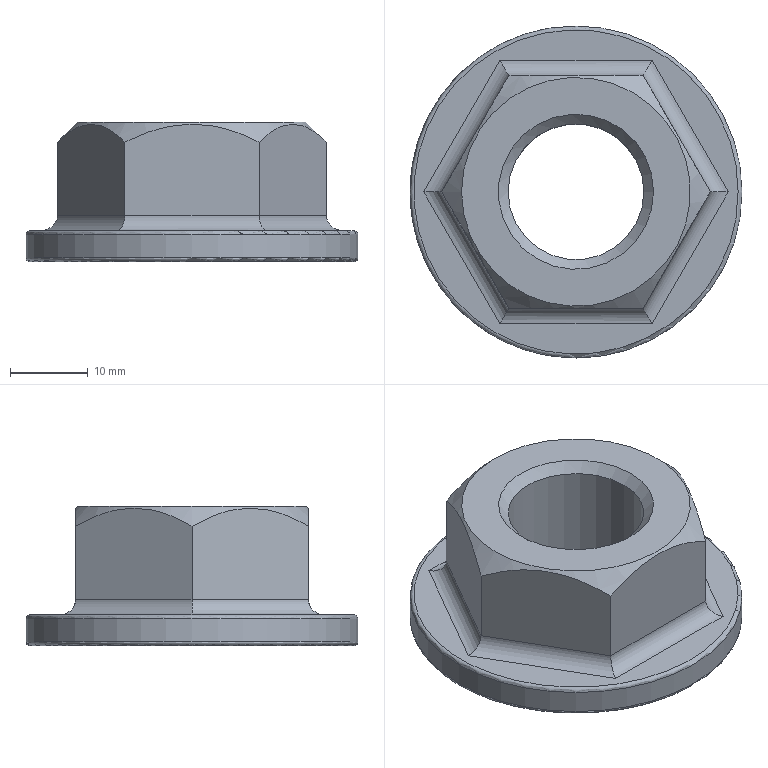Part | STEP file | 冲床-300配套压波_id1090_x_t | 1 solid | 22 faces | box 42.8 x 42.8 x 18 mm | volume 12253 mm3 | plane 9 | cylinder 8 | cone 3 | torus 2 | commonest cylinder face diameters 4 x6 17.5 x1 42.8 x1
STEP:
#1=CARTESIAN_POINT('',(1260.,-86.,317.));
#2=VERTEX_POINT('',#1);
#3=CARTESIAN_POINT('',(1250.,-86.,317.));
#4=DIRECTION('',(0.,0.,-1.));
#5=DIRECTION('',(1.,0.,0.));
#6=AXIS2_PLACEMENT_3D('',#3,#4,#5);
#7=CIRCLE('',#6,10.);
#8=EDGE_CURVE('',#2,#2,#7,.T.);
#9=ORIENTED_EDGE('',*,*,#8,.T.);
#10=EDGE_LOOP('',(#9));
#11=FACE_BOUND('',#10,.T.);
#12=CARTESIAN_POINT('',(1235.25,-86.,317.));
#13=VERTEX_POINT('',#12);
#14=CARTESIAN_POINT('',(1250.,-86.,317.));
#15=DIRECTION('',(0.,0.,1.));
#16=DIRECTION('',(-1.,0.,0.));
#17=AXIS2_PLACEMENT_3D('',#14,#15,#16);
#18=CIRCLE('',#17,14.75);
#19=EDGE_CURVE('',#13,#13,#18,.T.);
#20=ORIENTED_EDGE('',*,*,#19,.T.);
#21=EDGE_LOOP('',(#20));
#22=FACE_BOUND('',#21,.T.);
#23=CARTESIAN_POINT('',(1250.,-86.,317.));
#24=DIRECTION('',(0.,0.,1.));
#25=DIRECTION('',(1.,0.,0.));
#26=AXIS2_PLACEMENT_3D('',#23,#24,#25);
#27=PLANE('',#26);
#28=ADVANCED_FACE('',(#11,#22),#27,.T.);
#29=CARTESIAN_POINT('',(1270.9,-86.,303.));
#30=VERTEX_POINT('',#29);
#31=CARTESIAN_POINT('',(1250.,-86.,303.));
#32=DIRECTION('',(0.,0.,1.));
#33=DIRECTION('',(1.,0.,0.));
#34=AXIS2_PLACEMENT_3D('',#31,#32,#33);
#35=CIRCLE('',#34,20.9);
#36=EDGE_CURVE('',#30,#30,#35,.T.);
#37=ORIENTED_EDGE('',*,*,#36,.T.);
#38=EDGE_LOOP('',(#37));
#39=FACE_BOUND('',#38,.T.);
#40=CARTESIAN_POINT('',(1240.185,-103.,303.));
#41=VERTEX_POINT('',#40);
#42=CARTESIAN_POINT('',(1230.37,-86.,303.));
#43=VERTEX_POINT('',#42);
#44=CARTESIAN_POINT('',(1235.278,-94.5,303.));
#45=DIRECTION('',(-0.5,0.866,0.));
#46=VECTOR('',#45,1.);
#47=LINE('',#44,#46);
#48=EDGE_CURVE('',#41,#43,#47,.T.);
#49=ORIENTED_EDGE('',*,*,#48,.T.);
#50=CARTESIAN_POINT('',(1240.185,-69.,303.));
#51=VERTEX_POINT('',#50);
#52=CARTESIAN_POINT('',(1235.278,-77.5,303.));
#53=DIRECTION('',(0.5,0.866,0.));
#54=VECTOR('',#53,1.);
#55=LINE('',#52,#54);
#56=EDGE_CURVE('',#43,#51,#55,.T.);
#57=ORIENTED_EDGE('',*,*,#56,.T.);
#58=CARTESIAN_POINT('',(1259.815,-69.,303.));
#59=VERTEX_POINT('',#58);
#60=CARTESIAN_POINT('',(1250.,-69.,303.));
#61=DIRECTION('',(1.,0.,0.));
#62=VECTOR('',#61,1.);
#63=LINE('',#60,#62);
#64=EDGE_CURVE('',#51,#59,#63,.T.);
#65=ORIENTED_EDGE('',*,*,#64,.T.);
#66=CARTESIAN_POINT('',(1269.63,-86.,303.));
#67=VERTEX_POINT('',#66);
#68=CARTESIAN_POINT('',(1264.722,-77.5,303.));
#69=DIRECTION('',(0.5,-0.866,0.));
#70=VECTOR('',#69,1.);
#71=LINE('',#68,#70);
#72=EDGE_CURVE('',#59,#67,#71,.T.);
#73=ORIENTED_EDGE('',*,*,#72,.T.);
#74=CARTESIAN_POINT('',(1259.815,-103.,303.));
#75=VERTEX_POINT('',#74);
#76=CARTESIAN_POINT('',(1264.722,-94.5,303.));
#77=DIRECTION('',(-0.5,-0.866,0.));
#78=VECTOR('',#77,1.);
#79=LINE('',#76,#78);
#80=EDGE_CURVE('',#67,#75,#79,.T.);
#81=ORIENTED_EDGE('',*,*,#80,.T.);
#82=CARTESIAN_POINT('',(1250.,-103.,303.));
#83=DIRECTION('',(-1.,0.,0.));
#84=VECTOR('',#83,1.);
#85=LINE('',#82,#84);
#86=EDGE_CURVE('',#75,#41,#85,.T.);
#87=ORIENTED_EDGE('',*,*,#86,.T.);
#88=EDGE_LOOP('',(#49,#57,#65,#73,#81,#87));
#89=FACE_BOUND('',#88,.T.);
#90=CARTESIAN_POINT('',(1250.,-86.,303.));
#91=DIRECTION('',(0.,0.,1.));
#92=DIRECTION('',(1.,0.,0.));
#93=AXIS2_PLACEMENT_3D('',#90,#91,#92);
#94=PLANE('',#93);
#95=ADVANCED_FACE('',(#39,#89),#94,.T.);
#96=ORIENTED_EDGE('',*,*,#19,.F.);
#97=EDGE_LOOP('',(#96));
#98=FACE_BOUND('',#97,.T.);
#99=CARTESIAN_POINT('',(1258.66,-101.,314.429));
#100=VERTEX_POINT('',#99);
#101=CARTESIAN_POINT('',(1241.34,-101.,314.429));
#102=VERTEX_POINT('',#101);
#103=CARTESIAN_POINT('',(1258.66,-101.,314.429));
#104=CARTESIAN_POINT('',(1257.307,-101.,315.106));
#105=CARTESIAN_POINT('',(1255.923,-101.,315.681));
#106=CARTESIAN_POINT('',(1253.056,-101.,316.503));
#107=CARTESIAN_POINT('',(1251.544,-101.,316.747));
#108=CARTESIAN_POINT('',(1247.008,-101.,316.756));
#109=CARTESIAN_POINT('',(1244.062,-101.,315.791));
#110=CARTESIAN_POINT('',(1241.34,-101.,314.429));
#111=B_SPLINE_CURVE_WITH_KNOTS('',3,(#103,#104,#105,#106,#107,#108,#109,#110),.UNSPECIFIED.,.F.,.F.,(4,2,2,4),(0.,0.25,0.5,1.),.UNSPECIFIED.);
#112=EDGE_CURVE('',#100,#102,#111,.T.);
#113=ORIENTED_EDGE('',*,*,#112,.F.);
#114=CARTESIAN_POINT('',(1267.321,-86.,314.429));
#115=VERTEX_POINT('',#114);
#116=CARTESIAN_POINT('',(1267.321,-86.,314.429));
#117=CARTESIAN_POINT('',(1266.644,-87.172,315.106));
#118=CARTESIAN_POINT('',(1265.952,-88.37,315.681));
#119=CARTESIAN_POINT('',(1264.519,-90.853,316.503));
#120=CARTESIAN_POINT('',(1263.762,-92.163,316.747));
#121=CARTESIAN_POINT('',(1261.494,-96.091,316.756));
#122=CARTESIAN_POINT('',(1260.022,-98.642,315.791));
#123=CARTESIAN_POINT('',(1258.66,-101.,314.429));
#124=B_SPLINE_CURVE_WITH_KNOTS('',3,(#116,#117,#118,#119,#120,#121,#122,#123),.UNSPECIFIED.,.F.,.F.,(4,2,2,4),(0.,0.25,0.5,1.),.UNSPECIFIED.);
#125=EDGE_CURVE('',#115,#100,#124,.T.);
#126=ORIENTED_EDGE('',*,*,#125,.F.);
#127=CARTESIAN_POINT('',(1258.66,-71.,314.429));
#128=VERTEX_POINT('',#127);
#129=CARTESIAN_POINT('',(1258.66,-71.,314.429));
#130=CARTESIAN_POINT('',(1259.337,-72.172,315.106));
#131=CARTESIAN_POINT('',(1260.029,-73.37,315.681));
#132=CARTESIAN_POINT('',(1261.462,-75.853,316.503));
#133=CARTESIAN_POINT('',(1262.218,-77.163,316.747));
#134=CARTESIAN_POINT('',(1264.486,-81.091,316.756));
#135=CARTESIAN_POINT('',(1265.959,-83.642,315.791));
#136=CARTESIAN_POINT('',(1267.321,-86.,314.429));
#137=B_SPLINE_CURVE_WITH_KNOTS('',3,(#129,#130,#131,#132,#133,#134,#135,#136),.UNSPECIFIED.,.F.,.F.,(4,2,2,4),(0.,0.25,0.5,1.),.UNSPECIFIED.);
#138=EDGE_CURVE('',#128,#115,#137,.T.);
#139=ORIENTED_EDGE('',*,*,#138,.F.);
#140=CARTESIAN_POINT('',(1241.34,-71.,314.429));
#141=VERTEX_POINT('',#140);
#142=CARTESIAN_POINT('',(1241.34,-71.,314.429));
#143=CARTESIAN_POINT('',(1242.693,-71.,315.106));
#144=CARTESIAN_POINT('',(1244.077,-71.,315.681));
#145=CARTESIAN_POINT('',(1246.944,-71.,316.503));
#146=CARTESIAN_POINT('',(1248.456,-71.,316.747));
#147=CARTESIAN_POINT('',(1252.992,-71.,316.756));
#148=CARTESIAN_POINT('',(1255.938,-71.,315.791));
#149=CARTESIAN_POINT('',(1258.66,-71.,314.429));
#150=B_SPLINE_CURVE_WITH_KNOTS('',3,(#142,#143,#144,#145,#146,#147,#148,#149),.UNSPECIFIED.,.F.,.F.,(4,2,2,4),(0.,0.25,0.5,1.),.UNSPECIFIED.);
#151=EDGE_CURVE('',#141,#128,#150,.T.);
#152=ORIENTED_EDGE('',*,*,#151,.F.);
#153=CARTESIAN_POINT('',(1232.679,-86.,314.429));
#154=VERTEX_POINT('',#153);
#155=CARTESIAN_POINT('',(1232.679,-86.,314.429));
#156=CARTESIAN_POINT('',(1233.356,-84.828,315.106));
#157=CARTESIAN_POINT('',(1234.048,-83.63,315.681));
#158=CARTESIAN_POINT('',(1235.481,-81.147,316.503));
#159=CARTESIAN_POINT('',(1236.238,-79.837,316.747));
#160=CARTESIAN_POINT('',(1238.506,-75.909,316.756));
#161=CARTESIAN_POINT('',(1239.978,-73.358,315.791));
#162=CARTESIAN_POINT('',(1241.34,-71.,314.429));
#163=B_SPLINE_CURVE_WITH_KNOTS('',3,(#155,#156,#157,#158,#159,#160,#161,#162),.UNSPECIFIED.,.F.,.F.,(4,2,2,4),(0.,0.25,0.5,1.),.UNSPECIFIED.);
#164=EDGE_CURVE('',#154,#141,#163,.T.);
#165=ORIENTED_EDGE('',*,*,#164,.F.);
#166=CARTESIAN_POINT('',(1241.34,-101.,314.429));
#167=CARTESIAN_POINT('',(1240.663,-99.828,315.106));
#168=CARTESIAN_POINT('',(1239.971,-98.63,315.681));
#169=CARTESIAN_POINT('',(1238.538,-96.147,316.503));
#170=CARTESIAN_POINT('',(1237.782,-94.837,316.747));
#171=CARTESIAN_POINT('',(1235.514,-90.909,316.756));
#172=CARTESIAN_POINT('',(1234.041,-88.358,315.791));
#173=CARTESIAN_POINT('',(1232.679,-86.,314.429));
#174=B_SPLINE_CURVE_WITH_KNOTS('',3,(#166,#167,#168,#169,#170,#171,#172,#173),.UNSPECIFIED.,.F.,.F.,(4,2,2,4),(0.,0.25,0.5,1.),.UNSPECIFIED.);
#175=EDGE_CURVE('',#102,#154,#174,.T.);
#176=ORIENTED_EDGE('',*,*,#175,.F.);
#177=EDGE_LOOP('',(#113,#126,#139,#152,#165,#176));
#178=FACE_BOUND('',#177,.T.);
#179=CARTESIAN_POINT('',(1250.,-86.,317.));
#180=DIRECTION('',(0.,0.,-1.));
#181=DIRECTION('',(-1.,0.,0.));
#182=AXIS2_PLACEMENT_3D('',#179,#180,#181);
#183=CONICAL_SURFACE('',#182,14.75,45.);
#184=ADVANCED_FACE('',(#98,#178),#183,.T.);
#185=CARTESIAN_POINT('',(1241.34,-71.,305.));
#186=VERTEX_POINT('',#185);
#187=CARTESIAN_POINT('',(1241.34,-71.,319.));
#188=DIRECTION('',(0.,0.,-1.));
#189=VECTOR('',#188,1.);
#190=LINE('',#187,#189);
#191=EDGE_CURVE('',#141,#186,#190,.T.);
#192=ORIENTED_EDGE('',*,*,#191,.T.);
#193=CARTESIAN_POINT('',(1232.679,-86.,305.));
#194=VERTEX_POINT('',#193);
#195=CARTESIAN_POINT('',(1241.34,-71.,305.));
#196=DIRECTION('',(-0.5,-0.866,0.));
#197=VECTOR('',#196,1.);
#198=LINE('',#195,#197);
#199=EDGE_CURVE('',#186,#194,#198,.T.);
#200=ORIENTED_EDGE('',*,*,#199,.T.);
#201=CARTESIAN_POINT('',(1232.679,-86.,319.));
#202=DIRECTION('',(0.,0.,-1.));
#203=VECTOR('',#202,1.);
#204=LINE('',#201,#203);
#205=EDGE_CURVE('',#154,#194,#204,.T.);
#206=ORIENTED_EDGE('',*,*,#205,.F.);
#207=ORIENTED_EDGE('',*,*,#164,.T.);
#208=EDGE_LOOP('',(#192,#200,#206,#207));
#209=FACE_OUTER_BOUND('',#208,.T.);
#210=CARTESIAN_POINT('',(1241.34,-71.,319.));
#211=DIRECTION('',(0.866,-0.5,0.));
#212=DIRECTION('',(0.5,0.866,0.));
#213=AXIS2_PLACEMENT_3D('',#210,#211,#212);
#214=PLANE('',#213);
#215=ADVANCED_FACE('',(#209),#214,.F.);
#216=CARTESIAN_POINT('',(1258.66,-71.,305.));
#217=VERTEX_POINT('',#216);
#218=CARTESIAN_POINT('',(1258.66,-71.,319.));
#219=DIRECTION('',(0.,0.,-1.));
#220=VECTOR('',#219,1.);
#221=LINE('',#218,#220);
#222=EDGE_CURVE('',#128,#217,#221,.T.);
#223=ORIENTED_EDGE('',*,*,#222,.T.);
#224=CARTESIAN_POINT('',(1258.66,-71.,305.));
#225=DIRECTION('',(-1.,0.,0.));
#226=VECTOR('',#225,1.);
#227=LINE('',#224,#226);
#228=EDGE_CURVE('',#217,#186,#227,.T.);
#229=ORIENTED_EDGE('',*,*,#228,.T.);
#230=ORIENTED_EDGE('',*,*,#191,.F.);
#231=ORIENTED_EDGE('',*,*,#151,.T.);
#232=EDGE_LOOP('',(#223,#229,#230,#231));
#233=FACE_OUTER_BOUND('',#232,.T.);
#234=CARTESIAN_POINT('',(1258.66,-71.,319.));
#235=DIRECTION('',(0.,-1.,0.));
#236=DIRECTION('',(1.,0.,0.));
#237=AXIS2_PLACEMENT_3D('',#234,#235,#236);
#238=PLANE('',#237);
#239=ADVANCED_FACE('',(#233),#238,.F.);
#240=CARTESIAN_POINT('',(1267.321,-86.,305.));
#241=VERTEX_POINT('',#240);
#242=CARTESIAN_POINT('',(1267.321,-86.,319.));
#243=DIRECTION('',(0.,0.,-1.));
#244=VECTOR('',#243,1.);
#245=LINE('',#242,#244);
#246=EDGE_CURVE('',#115,#241,#245,.T.);
#247=ORIENTED_EDGE('',*,*,#246,.T.);
#248=CARTESIAN_POINT('',(1267.321,-86.,305.));
#249=DIRECTION('',(-0.5,0.866,0.));
#250=VECTOR('',#249,1.);
#251=LINE('',#248,#250);
#252=EDGE_CURVE('',#241,#217,#251,.T.);
#253=ORIENTED_EDGE('',*,*,#252,.T.);
#254=ORIENTED_EDGE('',*,*,#222,.F.);
#255=ORIENTED_EDGE('',*,*,#138,.T.);
#256=EDGE_LOOP('',(#247,#253,#254,#255));
#257=FACE_OUTER_BOUND('',#256,.T.);
#258=CARTESIAN_POINT('',(1267.321,-86.,319.));
#259=DIRECTION('',(-0.866,-0.5,0.));
#260=DIRECTION('',(0.5,-0.866,0.));
#261=AXIS2_PLACEMENT_3D('',#258,#259,#260);
#262=PLANE('',#261);
#263=ADVANCED_FACE('',(#257),#262,.F.);
#264=CARTESIAN_POINT('',(1258.66,-101.,305.));
#265=VERTEX_POINT('',#264);
#266=CARTESIAN_POINT('',(1258.66,-101.,319.));
#267=DIRECTION('',(0.,0.,-1.));
#268=VECTOR('',#267,1.);
#269=LINE('',#266,#268);
#270=EDGE_CURVE('',#100,#265,#269,.T.);
#271=ORIENTED_EDGE('',*,*,#270,.T.);
#272=CARTESIAN_POINT('',(1258.66,-101.,305.));
#273=DIRECTION('',(0.5,0.866,0.));
#274=VECTOR('',#273,1.);
#275=LINE('',#272,#274);
#276=EDGE_CURVE('',#265,#241,#275,.T.);
#277=ORIENTED_EDGE('',*,*,#276,.T.);
#278=ORIENTED_EDGE('',*,*,#246,.F.);
#279=ORIENTED_EDGE('',*,*,#125,.T.);
#280=EDGE_LOOP('',(#271,#277,#278,#279));
#281=FACE_OUTER_BOUND('',#280,.T.);
#282=CARTESIAN_POINT('',(1258.66,-101.,319.));
#283=DIRECTION('',(-0.866,0.5,0.));
#284=DIRECTION('',(-0.5,-0.866,0.));
#285=AXIS2_PLACEMENT_3D('',#282,#283,#284);
#286=PLANE('',#285);
#287=ADVANCED_FACE('',(#281),#286,.F.);
#288=CARTESIAN_POINT('',(1241.34,-101.,305.));
#289=VERTEX_POINT('',#288);
#290=CARTESIAN_POINT('',(1241.34,-101.,319.));
#291=DIRECTION('',(0.,0.,-1.));
#292=VECTOR('',#291,1.);
#293=LINE('',#290,#292);
#294=EDGE_CURVE('',#102,#289,#293,.T.);
#295=ORIENTED_EDGE('',*,*,#294,.T.);
#296=CARTESIAN_POINT('',(1241.34,-101.,305.));
#297=DIRECTION('',(1.,0.,0.));
#298=VECTOR('',#297,1.);
#299=LINE('',#296,#298);
#300=EDGE_CURVE('',#289,#265,#299,.T.);
#301=ORIENTED_EDGE('',*,*,#300,.T.);
#302=ORIENTED_EDGE('',*,*,#270,.F.);
#303=ORIENTED_EDGE('',*,*,#112,.T.);
#304=EDGE_LOOP('',(#295,#301,#302,#303));
#305=FACE_OUTER_BOUND('',#304,.T.);
#306=CARTESIAN_POINT('',(1241.34,-101.,319.));
#307=DIRECTION('',(0.,1.,0.));
#308=DIRECTION('',(-1.,0.,0.));
#309=AXIS2_PLACEMENT_3D('',#306,#307,#308);
#310=PLANE('',#309);
#311=ADVANCED_FACE('',(#305),#310,.F.);
#312=ORIENTED_EDGE('',*,*,#205,.T.);
#313=CARTESIAN_POINT('',(1232.679,-86.,305.));
#314=DIRECTION('',(0.5,-0.866,0.));
#315=VECTOR('',#314,1.);
#316=LINE('',#313,#315);
#317=EDGE_CURVE('',#194,#289,#316,.T.);
#318=ORIENTED_EDGE('',*,*,#317,.T.);
#319=ORIENTED_EDGE('',*,*,#294,.F.);
#320=ORIENTED_EDGE('',*,*,#175,.T.);
#321=EDGE_LOOP('',(#312,#318,#319,#320));
#322=FACE_OUTER_BOUND('',#321,.T.);
#323=CARTESIAN_POINT('',(1232.679,-86.,319.));
#324=DIRECTION('',(0.866,0.5,0.));
#325=DIRECTION('',(-0.5,0.866,0.));
#326=AXIS2_PLACEMENT_3D('',#323,#324,#325);
#327=PLANE('',#326);
#328=ADVANCED_FACE('',(#322),#327,.F.);
#329=CARTESIAN_POINT('',(1260.,-86.,299.));
#330=VERTEX_POINT('',#329);
#331=CARTESIAN_POINT('',(1250.,-86.,299.));
#332=DIRECTION('',(0.,0.,1.));
#333=DIRECTION('',(1.,0.,0.));
#334=AXIS2_PLACEMENT_3D('',#331,#332,#333);
#335=CIRCLE('',#334,10.);
#336=EDGE_CURVE('',#330,#330,#335,.T.);
#337=ORIENTED_EDGE('',*,*,#336,.T.);
#338=EDGE_LOOP('',(#337));
#339=FACE_BOUND('',#338,.T.);
#340=CARTESIAN_POINT('',(1270.9,-86.,299.));
#341=VERTEX_POINT('',#340);
#342=CARTESIAN_POINT('',(1250.,-86.,299.));
#343=DIRECTION('',(0.,0.,-1.));
#344=DIRECTION('',(1.,0.,0.));
#345=AXIS2_PLACEMENT_3D('',#342,#343,#344);
#346=CIRCLE('',#345,20.9);
#347=EDGE_CURVE('',#341,#341,#346,.T.);
#348=ORIENTED_EDGE('',*,*,#347,.T.);
#349=EDGE_LOOP('',(#348));
#350=FACE_BOUND('',#349,.T.);
#351=CARTESIAN_POINT('',(1250.,-86.,299.));
#352=DIRECTION('',(0.,0.,1.));
#353=DIRECTION('',(1.,0.,0.));
#354=AXIS2_PLACEMENT_3D('',#351,#352,#353);
#355=PLANE('',#354);
#356=ADVANCED_FACE('',(#339,#350),#355,.F.);
#357=CARTESIAN_POINT('',(1271.4,-86.,299.5));
#358=VERTEX_POINT('',#357);
#359=CARTESIAN_POINT('',(1250.,-86.,299.5));
#360=DIRECTION('',(0.,0.,1.));
#361=DIRECTION('',(1.,0.,0.));
#362=AXIS2_PLACEMENT_3D('',#359,#360,#361);
#363=CIRCLE('',#362,21.4);
#364=EDGE_CURVE('',#358,#358,#363,.T.);
#365=ORIENTED_EDGE('',*,*,#364,.T.);
#366=EDGE_LOOP('',(#365));
#367=FACE_BOUND('',#366,.T.);
#368=CARTESIAN_POINT('',(1271.4,-86.,302.5));
#369=VERTEX_POINT('',#368);
#370=CARTESIAN_POINT('',(1250.,-86.,302.5));
#371=DIRECTION('',(0.,0.,-1.));
#372=DIRECTION('',(1.,0.,0.));
#373=AXIS2_PLACEMENT_3D('',#370,#371,#372);
#374=CIRCLE('',#373,21.4);
#375=EDGE_CURVE('',#369,#369,#374,.T.);
#376=ORIENTED_EDGE('',*,*,#375,.T.);
#377=EDGE_LOOP('',(#376));
#378=FACE_BOUND('',#377,.T.);
#379=CARTESIAN_POINT('',(1250.,-86.,302.));
#380=DIRECTION('',(0.,0.,-1.));
#381=DIRECTION('',(-1.,0.,0.));
#382=AXIS2_PLACEMENT_3D('',#379,#380,#381);
#383=CYLINDRICAL_SURFACE('',#382,21.4);
#384=ADVANCED_FACE('',(#367,#378),#383,.T.);
#385=CARTESIAN_POINT('',(1240.185,-103.,305.));
#386=DIRECTION('',(0.866,-0.5,0.));
#387=DIRECTION('',(0.5,0.866,0.));
#388=AXIS2_PLACEMENT_3D('',#385,#386,#387);
#389=ELLIPSE('',#388,2.309,2.);
#390=EDGE_CURVE('',#41,#289,#389,.T.);
#391=ORIENTED_EDGE('',*,*,#390,.F.);
#392=ORIENTED_EDGE('',*,*,#86,.F.);
#393=CARTESIAN_POINT('',(1259.815,-103.,305.));
#394=DIRECTION('',(-0.866,-0.5,0.));
#395=DIRECTION('',(0.5,-0.866,0.));
#396=AXIS2_PLACEMENT_3D('',#393,#394,#395);
#397=ELLIPSE('',#396,2.309,2.);
#398=EDGE_CURVE('',#265,#75,#397,.T.);
#399=ORIENTED_EDGE('',*,*,#398,.F.);
#400=ORIENTED_EDGE('',*,*,#300,.F.);
#401=EDGE_LOOP('',(#391,#392,#399,#400));
#402=FACE_OUTER_BOUND('',#401,.T.);
#403=CARTESIAN_POINT('',(1241.34,-103.,305.));
#404=DIRECTION('',(1.,0.,0.));
#405=DIRECTION('',(0.,1.,0.));
#406=AXIS2_PLACEMENT_3D('',#403,#404,#405);
#407=CYLINDRICAL_SURFACE('',#406,2.);
#408=ADVANCED_FACE('',(#402),#407,.F.);
#409=ORIENTED_EDGE('',*,*,#398,.T.);
#410=ORIENTED_EDGE('',*,*,#80,.F.);
#411=CARTESIAN_POINT('',(1269.63,-86.,305.));
#412=DIRECTION('',(0.,-1.,0.));
#413=DIRECTION('',(1.,0.,0.));
#414=AXIS2_PLACEMENT_3D('',#411,#412,#413);
#415=ELLIPSE('',#414,2.309,2.);
#416=EDGE_CURVE('',#241,#67,#415,.T.);
#417=ORIENTED_EDGE('',*,*,#416,.F.);
#418=ORIENTED_EDGE('',*,*,#276,.F.);
#419=EDGE_LOOP('',(#409,#410,#417,#418));
#420=FACE_OUTER_BOUND('',#419,.T.);
#421=CARTESIAN_POINT('',(1260.392,-102.,305.));
#422=DIRECTION('',(0.5,0.866,0.));
#423=DIRECTION('',(-0.866,0.5,0.));
#424=AXIS2_PLACEMENT_3D('',#421,#422,#423);
#425=CYLINDRICAL_SURFACE('',#424,2.);
#426=ADVANCED_FACE('',(#420),#425,.F.);
#427=ORIENTED_EDGE('',*,*,#390,.T.);
#428=ORIENTED_EDGE('',*,*,#317,.F.);
#429=CARTESIAN_POINT('',(1230.37,-86.,305.));
#430=DIRECTION('',(0.,-1.,0.));
#431=DIRECTION('',(-1.,0.,0.));
#432=AXIS2_PLACEMENT_3D('',#429,#430,#431);
#433=ELLIPSE('',#432,2.309,2.);
#434=EDGE_CURVE('',#43,#194,#433,.T.);
#435=ORIENTED_EDGE('',*,*,#434,.F.);
#436=ORIENTED_EDGE('',*,*,#48,.F.);
#437=EDGE_LOOP('',(#427,#428,#435,#436));
#438=FACE_OUTER_BOUND('',#437,.T.);
#439=CARTESIAN_POINT('',(1230.947,-87.,305.));
#440=DIRECTION('',(0.5,-0.866,0.));
#441=DIRECTION('',(0.866,0.5,0.));
#442=AXIS2_PLACEMENT_3D('',#439,#440,#441);
#443=CYLINDRICAL_SURFACE('',#442,2.);
#444=ADVANCED_FACE('',(#438),#443,.F.);
#445=ORIENTED_EDGE('',*,*,#416,.T.);
#446=ORIENTED_EDGE('',*,*,#72,.F.);
#447=CARTESIAN_POINT('',(1259.815,-69.,305.));
#448=DIRECTION('',(0.866,-0.5,0.));
#449=DIRECTION('',(0.5,0.866,0.));
#450=AXIS2_PLACEMENT_3D('',#447,#448,#449);
#451=ELLIPSE('',#450,2.309,2.);
#452=EDGE_CURVE('',#217,#59,#451,.T.);
#453=ORIENTED_EDGE('',*,*,#452,.F.);
#454=ORIENTED_EDGE('',*,*,#252,.F.);
#455=EDGE_LOOP('',(#445,#446,#453,#454));
#456=FACE_OUTER_BOUND('',#455,.T.);
#457=CARTESIAN_POINT('',(1269.053,-85.,305.));
#458=DIRECTION('',(-0.5,0.866,0.));
#459=DIRECTION('',(-0.866,-0.5,0.));
#460=AXIS2_PLACEMENT_3D('',#457,#458,#459);
#461=CYLINDRICAL_SURFACE('',#460,2.);
#462=ADVANCED_FACE('',(#456),#461,.F.);
#463=ORIENTED_EDGE('',*,*,#434,.T.);
#464=ORIENTED_EDGE('',*,*,#199,.F.);
#465=CARTESIAN_POINT('',(1240.185,-69.,305.));
#466=DIRECTION('',(-0.866,-0.5,0.));
#467=DIRECTION('',(0.5,-0.866,0.));
#468=AXIS2_PLACEMENT_3D('',#465,#466,#467);
#469=ELLIPSE('',#468,2.309,2.);
#470=EDGE_CURVE('',#51,#186,#469,.T.);
#471=ORIENTED_EDGE('',*,*,#470,.F.);
#472=ORIENTED_EDGE('',*,*,#56,.F.);
#473=EDGE_LOOP('',(#463,#464,#471,#472));
#474=FACE_OUTER_BOUND('',#473,.T.);
#475=CARTESIAN_POINT('',(1239.608,-70.,305.));
#476=DIRECTION('',(-0.5,-0.866,0.));
#477=DIRECTION('',(0.866,-0.5,0.));
#478=AXIS2_PLACEMENT_3D('',#475,#476,#477);
#479=CYLINDRICAL_SURFACE('',#478,2.);
#480=ADVANCED_FACE('',(#474),#479,.F.);
#481=ORIENTED_EDGE('',*,*,#452,.T.);
#482=ORIENTED_EDGE('',*,*,#64,.F.);
#483=ORIENTED_EDGE('',*,*,#470,.T.);
#484=ORIENTED_EDGE('',*,*,#228,.F.);
#485=EDGE_LOOP('',(#481,#482,#483,#484));
#486=FACE_OUTER_BOUND('',#485,.T.);
#487=CARTESIAN_POINT('',(1258.66,-69.,305.));
#488=DIRECTION('',(-1.,0.,0.));
#489=DIRECTION('',(0.,-1.,0.));
#490=AXIS2_PLACEMENT_3D('',#487,#488,#489);
#491=CYLINDRICAL_SURFACE('',#490,2.);
#492=ADVANCED_FACE('',(#486),#491,.F.);
#493=ORIENTED_EDGE('',*,*,#364,.F.);
#494=EDGE_LOOP('',(#493));
#495=FACE_BOUND('',#494,.T.);
#496=ORIENTED_EDGE('',*,*,#347,.F.);
#497=EDGE_LOOP('',(#496));
#498=FACE_BOUND('',#497,.T.);
#499=CARTESIAN_POINT('',(1250.,-86.,299.5));
#500=DIRECTION('',(0.,0.,1.));
#501=DIRECTION('',(1.,0.,0.));
#502=AXIS2_PLACEMENT_3D('',#499,#500,#501);
#503=TOROIDAL_SURFACE('',#502,20.9,0.5);
#504=ADVANCED_FACE('',(#495,#498),#503,.T.);
#505=ORIENTED_EDGE('',*,*,#36,.F.);
#506=EDGE_LOOP('',(#505));
#507=FACE_BOUND('',#506,.T.);
#508=ORIENTED_EDGE('',*,*,#375,.F.);
#509=EDGE_LOOP('',(#508));
#510=FACE_BOUND('',#509,.T.);
#511=CARTESIAN_POINT('',(1250.,-86.,302.5));
#512=DIRECTION('',(0.,0.,1.));
#513=DIRECTION('',(1.,0.,0.));
#514=AXIS2_PLACEMENT_3D('',#511,#512,#513);
#515=TOROIDAL_SURFACE('',#514,20.9,0.5);
#516=ADVANCED_FACE('',(#507,#510),#515,.T.);
#517=CARTESIAN_POINT('',(1241.25,-86.,300.25));
#518=VERTEX_POINT('',#517);
#519=CARTESIAN_POINT('',(1250.,-86.,300.25));
#520=DIRECTION('',(0.,0.,-1.));
#521=DIRECTION('',(-1.,0.,0.));
#522=AXIS2_PLACEMENT_3D('',#519,#520,#521);
#523=CIRCLE('',#522,8.75);
#524=EDGE_CURVE('',#518,#518,#523,.T.);
#525=ORIENTED_EDGE('',*,*,#524,.T.);
#526=EDGE_LOOP('',(#525));
#527=FACE_BOUND('',#526,.T.);
#528=CARTESIAN_POINT('',(1258.75,-86.,315.75));
#529=VERTEX_POINT('',#528);
#530=CARTESIAN_POINT('',(1250.,-86.,315.75));
#531=DIRECTION('',(0.,0.,1.));
#532=DIRECTION('',(1.,0.,0.));
#533=AXIS2_PLACEMENT_3D('',#530,#531,#532);
#534=CIRCLE('',#533,8.75);
#535=EDGE_CURVE('',#529,#529,#534,.T.);
#536=ORIENTED_EDGE('',*,*,#535,.T.);
#537=EDGE_LOOP('',(#536));
#538=FACE_BOUND('',#537,.T.);
#539=CARTESIAN_POINT('',(1250.,-86.,319.));
#540=DIRECTION('',(0.,0.,-1.));
#541=DIRECTION('',(-1.,0.,0.));
#542=AXIS2_PLACEMENT_3D('',#539,#540,#541);
#543=CYLINDRICAL_SURFACE('',#542,8.75);
#544=ADVANCED_FACE('',(#527,#538),#543,.F.);
#545=ORIENTED_EDGE('',*,*,#535,.F.);
#546=EDGE_LOOP('',(#545));
#547=FACE_BOUND('',#546,.T.);
#548=ORIENTED_EDGE('',*,*,#8,.F.);
#549=EDGE_LOOP('',(#548));
#550=FACE_BOUND('',#549,.T.);
#551=CARTESIAN_POINT('',(1250.,-86.,317.));
#552=DIRECTION('',(0.,0.,1.));
#553=DIRECTION('',(1.,0.,0.));
#554=AXIS2_PLACEMENT_3D('',#551,#552,#553);
#555=CONICAL_SURFACE('',#554,10.,45.);
#556=ADVANCED_FACE('',(#547,#550),#555,.F.);
#557=ORIENTED_EDGE('',*,*,#336,.F.);
#558=EDGE_LOOP('',(#557));
#559=FACE_BOUND('',#558,.T.);
#560=ORIENTED_EDGE('',*,*,#524,.F.);
#561=EDGE_LOOP('',(#560));
#562=FACE_BOUND('',#561,.T.);
#563=CARTESIAN_POINT('',(1250.,-86.,300.25));
#564=DIRECTION('',(0.,0.,-1.));
#565=DIRECTION('',(-1.,0.,0.));
#566=AXIS2_PLACEMENT_3D('',#563,#564,#565);
#567=CONICAL_SURFACE('',#566,8.75,45.);
#568=ADVANCED_FACE('',(#559,#562),#567,.F.);
#569=CLOSED_SHELL('',(#28,#95,#184,#215,#239,#263,#287,#311,#328,#356,#384,#408,#426,#444,#462,#480,#492,#504,#516,#544,#556,#568));
#570=MANIFOLD_SOLID_BREP('',#569);
#571=(LENGTH_UNIT()NAMED_UNIT(*)SI_UNIT(.MILLI.,.METRE.));
#572=UNCERTAINTY_MEASURE_WITH_UNIT(LENGTH_MEASURE(0.0508),#571,'','');
#573=(NAMED_UNIT(*)PLANE_ANGLE_UNIT()SI_UNIT($,.RADIAN.));
#574=PLANE_ANGLE_MEASURE_WITH_UNIT(PLANE_ANGLE_MEASURE(0.01745),#573);
#575=DIMENSIONAL_EXPONENTS(0.,0.,0.,0.,0.,0.,0.);
#576=(CONVERSION_BASED_UNIT('DEGREE',#574)NAMED_UNIT(#575)PLANE_ANGLE_UNIT());
#577=(NAMED_UNIT(*)SI_UNIT($,.STERADIAN.)SOLID_ANGLE_UNIT());
#578=(GEOMETRIC_REPRESENTATION_CONTEXT(3)GLOBAL_UNCERTAINTY_ASSIGNED_CONTEXT((#572))GLOBAL_UNIT_ASSIGNED_CONTEXT((#571,#576,#577))REPRESENTATION_CONTEXT('',''));
#579=ADVANCED_BREP_SHAPE_REPRESENTATION('',(#570),#578);